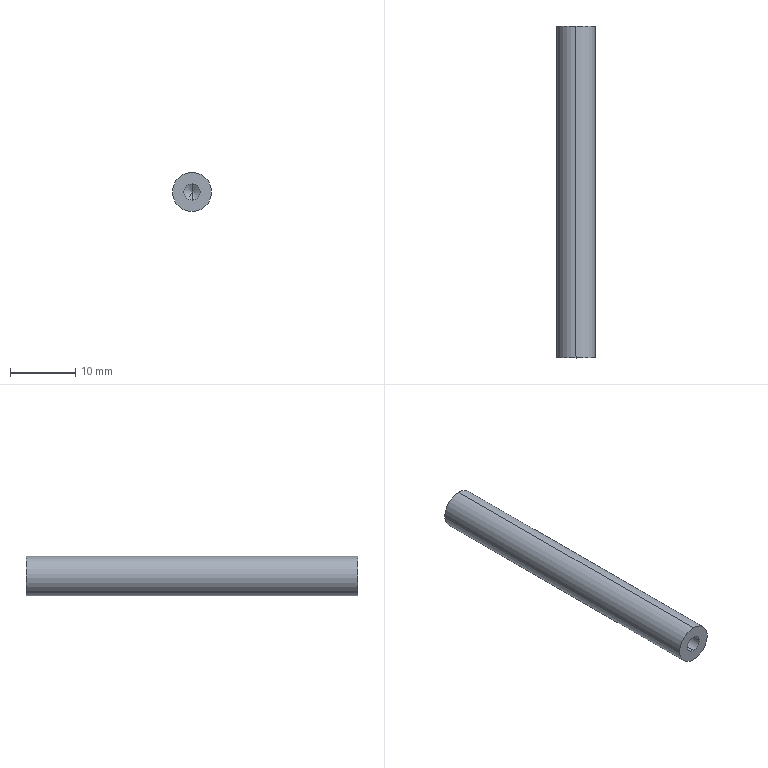Part | SolidWorks | features HoleWzd 2, BaseBody 1 | 1 solid | 12 faces | box 6 x 51 x 6 mm | volume 1381 mm3 | cylinder 6 | cone 4 | plane 2 | commonest cylinder face diameters 2.5 x4 6 x2
STEP:
#1=CARTESIAN_POINT('',(0.,45.,-1.25));
#2=VERTEX_POINT('',#1);
#3=CARTESIAN_POINT('',(0.,45.,1.25));
#4=VERTEX_POINT('',#3);
#5=CARTESIAN_POINT('',(0.,45.,0.));
#6=DIRECTION('',(0.,1.,0.));
#7=DIRECTION('',(0.,0.,1.));
#8=AXIS2_PLACEMENT_3D('',#5,#6,#7);
#9=CIRCLE('',#8,1.25);
#10=EDGE_CURVE('',#2,#4,#9,.T.);
#11=ORIENTED_EDGE('',*,*,#10,.F.);
#12=CARTESIAN_POINT('',(0.,51.,-1.25));
#13=VERTEX_POINT('',#12);
#14=CARTESIAN_POINT('',(0.,51.,-1.25));
#15=DIRECTION('',(0.,1.,0.));
#16=VECTOR('',#15,1000.);
#17=LINE('',#14,#16);
#18=EDGE_CURVE('',#2,#13,#17,.T.);
#19=ORIENTED_EDGE('',*,*,#18,.T.);
#20=CARTESIAN_POINT('',(0.,51.,1.25));
#21=VERTEX_POINT('',#20);
#22=CARTESIAN_POINT('',(0.,51.,0.));
#23=DIRECTION('',(0.,1.,0.));
#24=DIRECTION('',(0.,0.,1.));
#25=AXIS2_PLACEMENT_3D('',#22,#23,#24);
#26=CIRCLE('',#25,1.25);
#27=EDGE_CURVE('',#13,#21,#26,.T.);
#28=ORIENTED_EDGE('',*,*,#27,.T.);
#29=CARTESIAN_POINT('',(0.,51.,1.25));
#30=DIRECTION('',(0.,1.,0.));
#31=VECTOR('',#30,1000.);
#32=LINE('',#29,#31);
#33=EDGE_CURVE('',#4,#21,#32,.T.);
#34=ORIENTED_EDGE('',*,*,#33,.F.);
#35=EDGE_LOOP('',(#11,#19,#28,#34));
#36=FACE_OUTER_BOUND('',#35,.T.);
#37=CARTESIAN_POINT('',(0.,51.,0.));
#38=DIRECTION('',(0.,1.,0.));
#39=DIRECTION('',(0.,0.,1.));
#40=AXIS2_PLACEMENT_3D('',#37,#38,#39);
#41=CYLINDRICAL_SURFACE('',#40,1.25);
#42=ADVANCED_FACE('',(#36),#41,.F.);
#43=CARTESIAN_POINT('',(0.,44.249,0.));
#44=VERTEX_POINT('',#43);
#45=CARTESIAN_POINT('',(0.,45.,1.25));
#46=DIRECTION('',(0.,0.515,0.8572));
#47=VECTOR('',#46,1000.);
#48=LINE('',#45,#47);
#49=EDGE_CURVE('',#44,#4,#48,.T.);
#50=ORIENTED_EDGE('',*,*,#49,.F.);
#51=CARTESIAN_POINT('',(0.,45.,-1.25));
#52=DIRECTION('',(0.,0.515,-0.8572));
#53=VECTOR('',#52,1000.);
#54=LINE('',#51,#53);
#55=EDGE_CURVE('',#44,#2,#54,.T.);
#56=ORIENTED_EDGE('',*,*,#55,.T.);
#57=ORIENTED_EDGE('',*,*,#10,.T.);
#58=EDGE_LOOP('',(#50,#56,#57));
#59=FACE_OUTER_BOUND('',#58,.T.);
#60=CARTESIAN_POINT('',(0.,45.,0.));
#61=DIRECTION('',(0.,1.,0.));
#62=DIRECTION('',(0.,0.,1.));
#63=AXIS2_PLACEMENT_3D('',#60,#61,#62);
#64=CONICAL_SURFACE('',#63,1.25,1.03);
#65=ADVANCED_FACE('',(#59),#64,.F.);
#66=CARTESIAN_POINT('',(0.,6.,1.25));
#67=VERTEX_POINT('',#66);
#68=CARTESIAN_POINT('',(0.,6.,-1.25));
#69=VERTEX_POINT('',#68);
#70=CARTESIAN_POINT('',(0.,6.,0.));
#71=DIRECTION('',(0.,-1.,0.));
#72=DIRECTION('',(0.,0.,-1.));
#73=AXIS2_PLACEMENT_3D('',#70,#71,#72);
#74=CIRCLE('',#73,1.25);
#75=EDGE_CURVE('',#67,#69,#74,.T.);
#76=ORIENTED_EDGE('',*,*,#75,.F.);
#77=CARTESIAN_POINT('',(0.,0.,1.25));
#78=VERTEX_POINT('',#77);
#79=CARTESIAN_POINT('',(0.,0.,1.25));
#80=DIRECTION('',(0.,-1.,0.));
#81=VECTOR('',#80,1000.);
#82=LINE('',#79,#81);
#83=EDGE_CURVE('',#67,#78,#82,.T.);
#84=ORIENTED_EDGE('',*,*,#83,.T.);
#85=CARTESIAN_POINT('',(0.,0.,-1.25));
#86=VERTEX_POINT('',#85);
#87=CARTESIAN_POINT('',(0.,0.,0.));
#88=DIRECTION('',(0.,-1.,0.));
#89=DIRECTION('',(0.,0.,-1.));
#90=AXIS2_PLACEMENT_3D('',#87,#88,#89);
#91=CIRCLE('',#90,1.25);
#92=EDGE_CURVE('',#78,#86,#91,.T.);
#93=ORIENTED_EDGE('',*,*,#92,.T.);
#94=CARTESIAN_POINT('',(0.,0.,-1.25));
#95=DIRECTION('',(0.,-1.,0.));
#96=VECTOR('',#95,1000.);
#97=LINE('',#94,#96);
#98=EDGE_CURVE('',#69,#86,#97,.T.);
#99=ORIENTED_EDGE('',*,*,#98,.F.);
#100=EDGE_LOOP('',(#76,#84,#93,#99));
#101=FACE_OUTER_BOUND('',#100,.T.);
#102=CARTESIAN_POINT('',(0.,0.,0.));
#103=DIRECTION('',(0.,-1.,0.));
#104=DIRECTION('',(0.,0.,-1.));
#105=AXIS2_PLACEMENT_3D('',#102,#103,#104);
#106=CYLINDRICAL_SURFACE('',#105,1.25);
#107=ADVANCED_FACE('',(#101),#106,.F.);
#108=CARTESIAN_POINT('',(0.,6.751,0.));
#109=VERTEX_POINT('',#108);
#110=CARTESIAN_POINT('',(0.,6.,-1.25));
#111=DIRECTION('',(0.,-0.515,-0.8572));
#112=VECTOR('',#111,1000.);
#113=LINE('',#110,#112);
#114=EDGE_CURVE('',#109,#69,#113,.T.);
#115=ORIENTED_EDGE('',*,*,#114,.F.);
#116=CARTESIAN_POINT('',(0.,6.,1.25));
#117=DIRECTION('',(0.,-0.515,0.8572));
#118=VECTOR('',#117,1000.);
#119=LINE('',#116,#118);
#120=EDGE_CURVE('',#109,#67,#119,.T.);
#121=ORIENTED_EDGE('',*,*,#120,.T.);
#122=ORIENTED_EDGE('',*,*,#75,.T.);
#123=EDGE_LOOP('',(#115,#121,#122));
#124=FACE_OUTER_BOUND('',#123,.T.);
#125=CARTESIAN_POINT('',(0.,6.,0.));
#126=DIRECTION('',(0.,-1.,0.));
#127=DIRECTION('',(0.,0.,-1.));
#128=AXIS2_PLACEMENT_3D('',#125,#126,#127);
#129=CONICAL_SURFACE('',#128,1.25,1.03);
#130=ADVANCED_FACE('',(#124),#129,.F.);
#131=CARTESIAN_POINT('',(0.,0.,0.));
#132=DIRECTION('',(0.,-1.,0.));
#133=DIRECTION('',(0.,0.,-1.));
#134=AXIS2_PLACEMENT_3D('',#131,#132,#133);
#135=CIRCLE('',#134,1.25);
#136=EDGE_CURVE('',#86,#78,#135,.T.);
#137=ORIENTED_EDGE('',*,*,#136,.F.);
#138=ORIENTED_EDGE('',*,*,#92,.F.);
#139=EDGE_LOOP('',(#137,#138));
#140=FACE_BOUND('',#139,.T.);
#141=CARTESIAN_POINT('',(0.,0.,-3.));
#142=VERTEX_POINT('',#141);
#143=CARTESIAN_POINT('',(0.,0.,3.));
#144=VERTEX_POINT('',#143);
#145=CARTESIAN_POINT('',(0.,0.,0.));
#146=DIRECTION('',(0.,1.,0.));
#147=DIRECTION('',(0.,0.,1.));
#148=AXIS2_PLACEMENT_3D('',#145,#146,#147);
#149=CIRCLE('',#148,3.);
#150=EDGE_CURVE('',#142,#144,#149,.T.);
#151=ORIENTED_EDGE('',*,*,#150,.F.);
#152=CARTESIAN_POINT('',(0.,0.,0.));
#153=DIRECTION('',(0.,1.,0.));
#154=DIRECTION('',(0.,0.,1.));
#155=AXIS2_PLACEMENT_3D('',#152,#153,#154);
#156=CIRCLE('',#155,3.);
#157=EDGE_CURVE('',#144,#142,#156,.T.);
#158=ORIENTED_EDGE('',*,*,#157,.F.);
#159=EDGE_LOOP('',(#151,#158));
#160=FACE_OUTER_BOUND('',#159,.T.);
#161=CARTESIAN_POINT('',(0.,0.,0.));
#162=DIRECTION('',(0.,1.,0.));
#163=DIRECTION('',(1.,0.,0.));
#164=AXIS2_PLACEMENT_3D('',#161,#162,#163);
#165=PLANE('',#164);
#166=ADVANCED_FACE('',(#140,#160),#165,.F.);
#167=CARTESIAN_POINT('',(0.,51.,0.));
#168=DIRECTION('',(0.,1.,0.));
#169=DIRECTION('',(0.,0.,1.));
#170=AXIS2_PLACEMENT_3D('',#167,#168,#169);
#171=CIRCLE('',#170,1.25);
#172=EDGE_CURVE('',#21,#13,#171,.T.);
#173=ORIENTED_EDGE('',*,*,#172,.F.);
#174=ORIENTED_EDGE('',*,*,#27,.F.);
#175=EDGE_LOOP('',(#173,#174));
#176=FACE_BOUND('',#175,.T.);
#177=CARTESIAN_POINT('',(0.,51.,-3.));
#178=VERTEX_POINT('',#177);
#179=CARTESIAN_POINT('',(0.,51.,3.));
#180=VERTEX_POINT('',#179);
#181=CARTESIAN_POINT('',(0.,51.,0.));
#182=DIRECTION('',(0.,1.,0.));
#183=DIRECTION('',(0.,0.,1.));
#184=AXIS2_PLACEMENT_3D('',#181,#182,#183);
#185=CIRCLE('',#184,3.);
#186=EDGE_CURVE('',#178,#180,#185,.T.);
#187=ORIENTED_EDGE('',*,*,#186,.T.);
#188=CARTESIAN_POINT('',(0.,51.,0.));
#189=DIRECTION('',(0.,1.,0.));
#190=DIRECTION('',(0.,0.,1.));
#191=AXIS2_PLACEMENT_3D('',#188,#189,#190);
#192=CIRCLE('',#191,3.);
#193=EDGE_CURVE('',#180,#178,#192,.T.);
#194=ORIENTED_EDGE('',*,*,#193,.T.);
#195=EDGE_LOOP('',(#187,#194));
#196=FACE_OUTER_BOUND('',#195,.T.);
#197=CARTESIAN_POINT('',(0.,51.,0.));
#198=DIRECTION('',(0.,1.,0.));
#199=DIRECTION('',(1.,0.,0.));
#200=AXIS2_PLACEMENT_3D('',#197,#198,#199);
#201=PLANE('',#200);
#202=ADVANCED_FACE('',(#176,#196),#201,.T.);
#203=CARTESIAN_POINT('',(0.,51.,3.));
#204=DIRECTION('',(0.,-1.,0.));
#205=VECTOR('',#204,1000.);
#206=LINE('',#203,#205);
#207=EDGE_CURVE('',#180,#144,#206,.T.);
#208=ORIENTED_EDGE('',*,*,#207,.F.);
#209=ORIENTED_EDGE('',*,*,#186,.F.);
#210=CARTESIAN_POINT('',(0.,51.,-3.));
#211=DIRECTION('',(0.,-1.,0.));
#212=VECTOR('',#211,1000.);
#213=LINE('',#210,#212);
#214=EDGE_CURVE('',#178,#142,#213,.T.);
#215=ORIENTED_EDGE('',*,*,#214,.T.);
#216=ORIENTED_EDGE('',*,*,#150,.T.);
#217=EDGE_LOOP('',(#208,#209,#215,#216));
#218=FACE_OUTER_BOUND('',#217,.T.);
#219=CARTESIAN_POINT('',(0.,51.,0.));
#220=DIRECTION('',(0.,-1.,0.));
#221=DIRECTION('',(0.,0.,-1.));
#222=AXIS2_PLACEMENT_3D('',#219,#220,#221);
#223=CYLINDRICAL_SURFACE('',#222,3.);
#224=ADVANCED_FACE('',(#218),#223,.T.);
#225=ORIENTED_EDGE('',*,*,#193,.F.);
#226=ORIENTED_EDGE('',*,*,#207,.T.);
#227=ORIENTED_EDGE('',*,*,#157,.T.);
#228=ORIENTED_EDGE('',*,*,#214,.F.);
#229=EDGE_LOOP('',(#225,#226,#227,#228));
#230=FACE_OUTER_BOUND('',#229,.T.);
#231=CARTESIAN_POINT('',(0.,51.,0.));
#232=DIRECTION('',(0.,-1.,0.));
#233=DIRECTION('',(0.,0.,-1.));
#234=AXIS2_PLACEMENT_3D('',#231,#232,#233);
#235=CYLINDRICAL_SURFACE('',#234,3.);
#236=ADVANCED_FACE('',(#230),#235,.T.);
#237=ORIENTED_EDGE('',*,*,#120,.F.);
#238=ORIENTED_EDGE('',*,*,#114,.T.);
#239=CARTESIAN_POINT('',(0.,6.,0.));
#240=DIRECTION('',(0.,-1.,0.));
#241=DIRECTION('',(0.,0.,-1.));
#242=AXIS2_PLACEMENT_3D('',#239,#240,#241);
#243=CIRCLE('',#242,1.25);
#244=EDGE_CURVE('',#69,#67,#243,.T.);
#245=ORIENTED_EDGE('',*,*,#244,.T.);
#246=EDGE_LOOP('',(#237,#238,#245));
#247=FACE_OUTER_BOUND('',#246,.T.);
#248=CARTESIAN_POINT('',(0.,6.,0.));
#249=DIRECTION('',(0.,-1.,0.));
#250=DIRECTION('',(0.,0.,-1.));
#251=AXIS2_PLACEMENT_3D('',#248,#249,#250);
#252=CONICAL_SURFACE('',#251,1.25,1.03);
#253=ADVANCED_FACE('',(#247),#252,.F.);
#254=ORIENTED_EDGE('',*,*,#83,.F.);
#255=ORIENTED_EDGE('',*,*,#244,.F.);
#256=ORIENTED_EDGE('',*,*,#98,.T.);
#257=ORIENTED_EDGE('',*,*,#136,.T.);
#258=EDGE_LOOP('',(#254,#255,#256,#257));
#259=FACE_OUTER_BOUND('',#258,.T.);
#260=CARTESIAN_POINT('',(0.,0.,0.));
#261=DIRECTION('',(0.,-1.,0.));
#262=DIRECTION('',(0.,0.,-1.));
#263=AXIS2_PLACEMENT_3D('',#260,#261,#262);
#264=CYLINDRICAL_SURFACE('',#263,1.25);
#265=ADVANCED_FACE('',(#259),#264,.F.);
#266=ORIENTED_EDGE('',*,*,#55,.F.);
#267=ORIENTED_EDGE('',*,*,#49,.T.);
#268=CARTESIAN_POINT('',(0.,45.,0.));
#269=DIRECTION('',(0.,1.,0.));
#270=DIRECTION('',(0.,0.,1.));
#271=AXIS2_PLACEMENT_3D('',#268,#269,#270);
#272=CIRCLE('',#271,1.25);
#273=EDGE_CURVE('',#4,#2,#272,.T.);
#274=ORIENTED_EDGE('',*,*,#273,.T.);
#275=EDGE_LOOP('',(#266,#267,#274));
#276=FACE_OUTER_BOUND('',#275,.T.);
#277=CARTESIAN_POINT('',(0.,45.,0.));
#278=DIRECTION('',(0.,1.,0.));
#279=DIRECTION('',(0.,0.,1.));
#280=AXIS2_PLACEMENT_3D('',#277,#278,#279);
#281=CONICAL_SURFACE('',#280,1.25,1.03);
#282=ADVANCED_FACE('',(#276),#281,.F.);
#283=ORIENTED_EDGE('',*,*,#18,.F.);
#284=ORIENTED_EDGE('',*,*,#273,.F.);
#285=ORIENTED_EDGE('',*,*,#33,.T.);
#286=ORIENTED_EDGE('',*,*,#172,.T.);
#287=EDGE_LOOP('',(#283,#284,#285,#286));
#288=FACE_OUTER_BOUND('',#287,.T.);
#289=CARTESIAN_POINT('',(0.,51.,0.));
#290=DIRECTION('',(0.,1.,0.));
#291=DIRECTION('',(0.,0.,1.));
#292=AXIS2_PLACEMENT_3D('',#289,#290,#291);
#293=CYLINDRICAL_SURFACE('',#292,1.25);
#294=ADVANCED_FACE('',(#288),#293,.F.);
#295=CLOSED_SHELL('',(#42,#65,#107,#130,#166,#202,#224,#236,#253,#265,#282,#294));
#296=MANIFOLD_SOLID_BREP('',#295);
#297=CARTESIAN_POINT('',(0.,0.,0.));
#298=DIRECTION('',(0.,0.,1.));
#299=DIRECTION('',(1.,0.,0.));
#300=AXIS2_PLACEMENT_3D('',#297,#298,#299);
#301=(LENGTH_UNIT()NAMED_UNIT(*)SI_UNIT(.MILLI.,.METRE.));
#302=UNCERTAINTY_MEASURE_WITH_UNIT(LENGTH_MEASURE(0.00001),#301,'','');
#303=(NAMED_UNIT(*)PLANE_ANGLE_UNIT()SI_UNIT($,.RADIAN.));
#304=(NAMED_UNIT(*)SI_UNIT($,.STERADIAN.)SOLID_ANGLE_UNIT());
#305=(GEOMETRIC_REPRESENTATION_CONTEXT(3)GLOBAL_UNCERTAINTY_ASSIGNED_CONTEXT((#302))GLOBAL_UNIT_ASSIGNED_CONTEXT((#301,#303,#304))REPRESENTATION_CONTEXT('',''));
#306=ADVANCED_BREP_SHAPE_REPRESENTATION('',(#296,#300),#305);